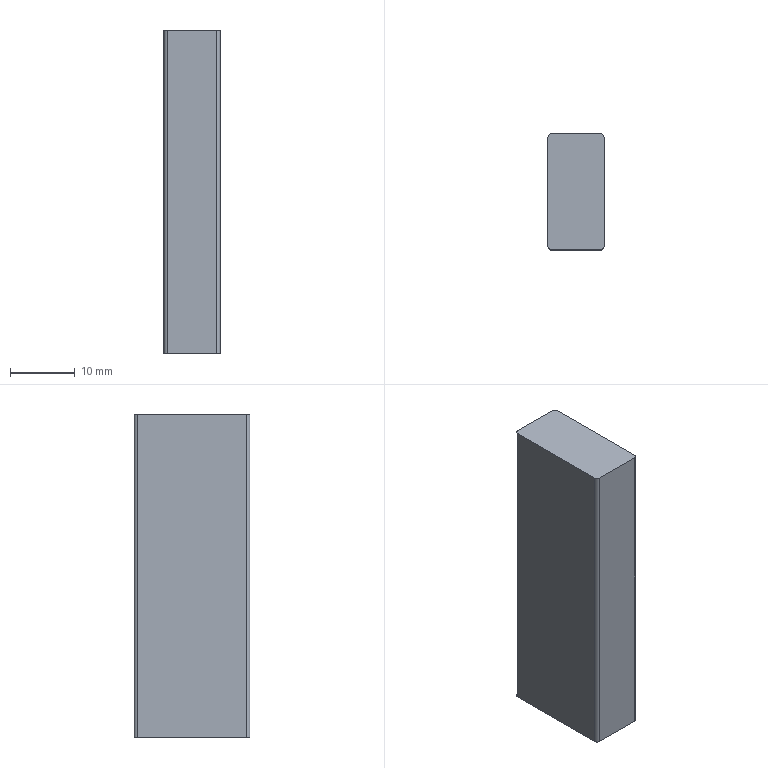Part | NX | features BREP 1 | 1 solid | 10 faces | box 8.68 x 17.946 x 50 mm | volume 7778 mm3 | plane 6 | cylinder 4 | commonest cylinder face diameters 1 x4
STEP:
#1=CARTESIAN_POINT('',(-3.84,8.973,-40.6));
#2=VERTEX_POINT('',#1);
#3=CARTESIAN_POINT('',(-4.34,8.473,-40.6));
#4=VERTEX_POINT('',#3);
#5=CARTESIAN_POINT('',(-3.84,8.473,-40.6));
#6=DIRECTION('',(0.,0.,1.));
#7=DIRECTION('',(1.,0.,0.));
#8=AXIS2_PLACEMENT_3D('',#5,#6,#7);
#9=CIRCLE('',#8,0.5);
#10=EDGE_CURVE('',#2,#4,#9,.T.);
#11=ORIENTED_EDGE('',*,*,#10,.F.);
#12=CARTESIAN_POINT('',(-3.84,8.973,-90.6));
#13=VERTEX_POINT('',#12);
#14=CARTESIAN_POINT('',(-3.84,8.973,-90.6));
#15=DIRECTION('',(0.,0.,1.));
#16=VECTOR('',#15,1000.);
#17=LINE('',#14,#16);
#18=EDGE_CURVE('',#13,#2,#17,.T.);
#19=ORIENTED_EDGE('',*,*,#18,.F.);
#20=CARTESIAN_POINT('',(-4.34,8.473,-90.6));
#21=VERTEX_POINT('',#20);
#22=CARTESIAN_POINT('',(-3.84,8.473,-90.6));
#23=DIRECTION('',(0.,0.,1.));
#24=DIRECTION('',(1.,0.,0.));
#25=AXIS2_PLACEMENT_3D('',#22,#23,#24);
#26=CIRCLE('',#25,0.5);
#27=EDGE_CURVE('',#13,#21,#26,.T.);
#28=ORIENTED_EDGE('',*,*,#27,.T.);
#29=CARTESIAN_POINT('',(-4.34,8.473,-90.6));
#30=DIRECTION('',(0.,0.,1.));
#31=VECTOR('',#30,1000.);
#32=LINE('',#29,#31);
#33=EDGE_CURVE('',#21,#4,#32,.T.);
#34=ORIENTED_EDGE('',*,*,#33,.T.);
#35=EDGE_LOOP('',(#11,#19,#28,#34));
#36=FACE_BOUND('',#35,.T.);
#37=CARTESIAN_POINT('',(-3.84,8.473,-90.6));
#38=DIRECTION('',(0.,0.,1.));
#39=DIRECTION('',(-1.,0.,0.));
#40=AXIS2_PLACEMENT_3D('',#37,#38,#39);
#41=CYLINDRICAL_SURFACE('',#40,0.5);
#42=ADVANCED_FACE('',(#36),#41,.T.);
#43=CARTESIAN_POINT('',(-4.34,-8.473,-40.6));
#44=VERTEX_POINT('',#43);
#45=CARTESIAN_POINT('',(-4.34,-8.473,-40.6));
#46=DIRECTION('',(0.,1.,0.));
#47=VECTOR('',#46,1000.);
#48=LINE('',#45,#47);
#49=EDGE_CURVE('',#44,#4,#48,.T.);
#50=ORIENTED_EDGE('',*,*,#49,.T.);
#51=ORIENTED_EDGE('',*,*,#33,.F.);
#52=CARTESIAN_POINT('',(-4.34,-8.473,-90.6));
#53=VERTEX_POINT('',#52);
#54=CARTESIAN_POINT('',(-4.34,-8.473,-90.6));
#55=DIRECTION('',(0.,1.,0.));
#56=VECTOR('',#55,1000.);
#57=LINE('',#54,#56);
#58=EDGE_CURVE('',#53,#21,#57,.T.);
#59=ORIENTED_EDGE('',*,*,#58,.F.);
#60=CARTESIAN_POINT('',(-4.34,-8.473,-90.6));
#61=DIRECTION('',(0.,0.,1.));
#62=VECTOR('',#61,1000.);
#63=LINE('',#60,#62);
#64=EDGE_CURVE('',#53,#44,#63,.T.);
#65=ORIENTED_EDGE('',*,*,#64,.T.);
#66=EDGE_LOOP('',(#50,#51,#59,#65));
#67=FACE_BOUND('',#66,.T.);
#68=CARTESIAN_POINT('',(-4.34,-8.473,-90.6));
#69=DIRECTION('',(1.,0.,0.));
#70=DIRECTION('',(0.,-1.,0.));
#71=AXIS2_PLACEMENT_3D('',#68,#69,#70);
#72=PLANE('',#71);
#73=ADVANCED_FACE('',(#67),#72,.F.);
#74=CARTESIAN_POINT('',(-3.84,-8.973,-40.6));
#75=VERTEX_POINT('',#74);
#76=CARTESIAN_POINT('',(-3.84,-8.473,-40.6));
#77=DIRECTION('',(0.,0.,1.));
#78=DIRECTION('',(1.,0.,0.));
#79=AXIS2_PLACEMENT_3D('',#76,#77,#78);
#80=CIRCLE('',#79,0.5);
#81=EDGE_CURVE('',#44,#75,#80,.T.);
#82=ORIENTED_EDGE('',*,*,#81,.F.);
#83=ORIENTED_EDGE('',*,*,#64,.F.);
#84=CARTESIAN_POINT('',(-3.84,-8.973,-90.6));
#85=VERTEX_POINT('',#84);
#86=CARTESIAN_POINT('',(-3.84,-8.473,-90.6));
#87=DIRECTION('',(0.,0.,1.));
#88=DIRECTION('',(1.,0.,0.));
#89=AXIS2_PLACEMENT_3D('',#86,#87,#88);
#90=CIRCLE('',#89,0.5);
#91=EDGE_CURVE('',#53,#85,#90,.T.);
#92=ORIENTED_EDGE('',*,*,#91,.T.);
#93=CARTESIAN_POINT('',(-3.84,-8.973,-90.6));
#94=DIRECTION('',(0.,0.,1.));
#95=VECTOR('',#94,1000.);
#96=LINE('',#93,#95);
#97=EDGE_CURVE('',#85,#75,#96,.T.);
#98=ORIENTED_EDGE('',*,*,#97,.T.);
#99=EDGE_LOOP('',(#82,#83,#92,#98));
#100=FACE_BOUND('',#99,.T.);
#101=CARTESIAN_POINT('',(-3.84,-8.473,-90.6));
#102=DIRECTION('',(0.,0.,1.));
#103=DIRECTION('',(-1.,0.,0.));
#104=AXIS2_PLACEMENT_3D('',#101,#102,#103);
#105=CYLINDRICAL_SURFACE('',#104,0.5);
#106=ADVANCED_FACE('',(#100),#105,.T.);
#107=CARTESIAN_POINT('',(3.84,-8.973,-40.6));
#108=VERTEX_POINT('',#107);
#109=CARTESIAN_POINT('',(3.84,-8.973,-40.6));
#110=DIRECTION('',(-1.,0.,0.));
#111=VECTOR('',#110,1000.);
#112=LINE('',#109,#111);
#113=EDGE_CURVE('',#108,#75,#112,.T.);
#114=ORIENTED_EDGE('',*,*,#113,.T.);
#115=ORIENTED_EDGE('',*,*,#97,.F.);
#116=CARTESIAN_POINT('',(3.84,-8.973,-90.6));
#117=VERTEX_POINT('',#116);
#118=CARTESIAN_POINT('',(3.84,-8.973,-90.6));
#119=DIRECTION('',(-1.,0.,0.));
#120=VECTOR('',#119,1000.);
#121=LINE('',#118,#120);
#122=EDGE_CURVE('',#117,#85,#121,.T.);
#123=ORIENTED_EDGE('',*,*,#122,.F.);
#124=CARTESIAN_POINT('',(3.84,-8.973,-90.6));
#125=DIRECTION('',(0.,0.,1.));
#126=VECTOR('',#125,1000.);
#127=LINE('',#124,#126);
#128=EDGE_CURVE('',#117,#108,#127,.T.);
#129=ORIENTED_EDGE('',*,*,#128,.T.);
#130=EDGE_LOOP('',(#114,#115,#123,#129));
#131=FACE_BOUND('',#130,.T.);
#132=CARTESIAN_POINT('',(3.84,-8.973,-90.6));
#133=DIRECTION('',(0.,1.,0.));
#134=DIRECTION('',(0.,0.,-1.));
#135=AXIS2_PLACEMENT_3D('',#132,#133,#134);
#136=PLANE('',#135);
#137=ADVANCED_FACE('',(#131),#136,.F.);
#138=CARTESIAN_POINT('',(4.34,-8.473,-40.6));
#139=VERTEX_POINT('',#138);
#140=CARTESIAN_POINT('',(3.84,-8.473,-40.6));
#141=DIRECTION('',(0.,0.,1.));
#142=DIRECTION('',(1.,0.,0.));
#143=AXIS2_PLACEMENT_3D('',#140,#141,#142);
#144=CIRCLE('',#143,0.5);
#145=EDGE_CURVE('',#108,#139,#144,.T.);
#146=ORIENTED_EDGE('',*,*,#145,.F.);
#147=ORIENTED_EDGE('',*,*,#128,.F.);
#148=CARTESIAN_POINT('',(4.34,-8.473,-90.6));
#149=VERTEX_POINT('',#148);
#150=CARTESIAN_POINT('',(3.84,-8.473,-90.6));
#151=DIRECTION('',(0.,0.,1.));
#152=DIRECTION('',(1.,0.,0.));
#153=AXIS2_PLACEMENT_3D('',#150,#151,#152);
#154=CIRCLE('',#153,0.5);
#155=EDGE_CURVE('',#117,#149,#154,.T.);
#156=ORIENTED_EDGE('',*,*,#155,.T.);
#157=CARTESIAN_POINT('',(4.34,-8.473,-90.6));
#158=DIRECTION('',(0.,0.,1.));
#159=VECTOR('',#158,1000.);
#160=LINE('',#157,#159);
#161=EDGE_CURVE('',#149,#139,#160,.T.);
#162=ORIENTED_EDGE('',*,*,#161,.T.);
#163=EDGE_LOOP('',(#146,#147,#156,#162));
#164=FACE_BOUND('',#163,.T.);
#165=CARTESIAN_POINT('',(3.84,-8.473,-90.6));
#166=DIRECTION('',(0.,0.,1.));
#167=DIRECTION('',(-1.,0.,0.));
#168=AXIS2_PLACEMENT_3D('',#165,#166,#167);
#169=CYLINDRICAL_SURFACE('',#168,0.5);
#170=ADVANCED_FACE('',(#164),#169,.T.);
#171=CARTESIAN_POINT('',(4.34,8.473,-40.6));
#172=VERTEX_POINT('',#171);
#173=CARTESIAN_POINT('',(4.34,8.473,-40.6));
#174=DIRECTION('',(0.,-1.,0.));
#175=VECTOR('',#174,1000.);
#176=LINE('',#173,#175);
#177=EDGE_CURVE('',#172,#139,#176,.T.);
#178=ORIENTED_EDGE('',*,*,#177,.T.);
#179=ORIENTED_EDGE('',*,*,#161,.F.);
#180=CARTESIAN_POINT('',(4.34,8.473,-90.6));
#181=VERTEX_POINT('',#180);
#182=CARTESIAN_POINT('',(4.34,8.473,-90.6));
#183=DIRECTION('',(0.,-1.,0.));
#184=VECTOR('',#183,1000.);
#185=LINE('',#182,#184);
#186=EDGE_CURVE('',#181,#149,#185,.T.);
#187=ORIENTED_EDGE('',*,*,#186,.F.);
#188=CARTESIAN_POINT('',(4.34,8.473,-90.6));
#189=DIRECTION('',(0.,0.,1.));
#190=VECTOR('',#189,1000.);
#191=LINE('',#188,#190);
#192=EDGE_CURVE('',#181,#172,#191,.T.);
#193=ORIENTED_EDGE('',*,*,#192,.T.);
#194=EDGE_LOOP('',(#178,#179,#187,#193));
#195=FACE_BOUND('',#194,.T.);
#196=CARTESIAN_POINT('',(4.34,8.473,-90.6));
#197=DIRECTION('',(-1.,0.,0.));
#198=DIRECTION('',(0.,0.,-1.));
#199=AXIS2_PLACEMENT_3D('',#196,#197,#198);
#200=PLANE('',#199);
#201=ADVANCED_FACE('',(#195),#200,.F.);
#202=CARTESIAN_POINT('',(3.84,8.973,-40.6));
#203=VERTEX_POINT('',#202);
#204=CARTESIAN_POINT('',(3.84,8.473,-40.6));
#205=DIRECTION('',(0.,0.,1.));
#206=DIRECTION('',(1.,0.,0.));
#207=AXIS2_PLACEMENT_3D('',#204,#205,#206);
#208=CIRCLE('',#207,0.5);
#209=EDGE_CURVE('',#172,#203,#208,.T.);
#210=ORIENTED_EDGE('',*,*,#209,.F.);
#211=ORIENTED_EDGE('',*,*,#192,.F.);
#212=CARTESIAN_POINT('',(3.84,8.973,-90.6));
#213=VERTEX_POINT('',#212);
#214=CARTESIAN_POINT('',(3.84,8.473,-90.6));
#215=DIRECTION('',(0.,0.,1.));
#216=DIRECTION('',(1.,0.,0.));
#217=AXIS2_PLACEMENT_3D('',#214,#215,#216);
#218=CIRCLE('',#217,0.5);
#219=EDGE_CURVE('',#181,#213,#218,.T.);
#220=ORIENTED_EDGE('',*,*,#219,.T.);
#221=CARTESIAN_POINT('',(3.84,8.973,-90.6));
#222=DIRECTION('',(0.,0.,1.));
#223=VECTOR('',#222,1000.);
#224=LINE('',#221,#223);
#225=EDGE_CURVE('',#213,#203,#224,.T.);
#226=ORIENTED_EDGE('',*,*,#225,.T.);
#227=EDGE_LOOP('',(#210,#211,#220,#226));
#228=FACE_BOUND('',#227,.T.);
#229=CARTESIAN_POINT('',(3.84,8.473,-90.6));
#230=DIRECTION('',(0.,0.,1.));
#231=DIRECTION('',(-1.,0.,0.));
#232=AXIS2_PLACEMENT_3D('',#229,#230,#231);
#233=CYLINDRICAL_SURFACE('',#232,0.5);
#234=ADVANCED_FACE('',(#228),#233,.T.);
#235=CARTESIAN_POINT('',(-3.84,8.973,-40.6));
#236=DIRECTION('',(1.,0.,0.));
#237=VECTOR('',#236,1000.);
#238=LINE('',#235,#237);
#239=EDGE_CURVE('',#2,#203,#238,.T.);
#240=ORIENTED_EDGE('',*,*,#239,.T.);
#241=ORIENTED_EDGE('',*,*,#225,.F.);
#242=CARTESIAN_POINT('',(-3.84,8.973,-90.6));
#243=DIRECTION('',(1.,0.,0.));
#244=VECTOR('',#243,1000.);
#245=LINE('',#242,#244);
#246=EDGE_CURVE('',#13,#213,#245,.T.);
#247=ORIENTED_EDGE('',*,*,#246,.F.);
#248=ORIENTED_EDGE('',*,*,#18,.T.);
#249=EDGE_LOOP('',(#240,#241,#247,#248));
#250=FACE_BOUND('',#249,.T.);
#251=CARTESIAN_POINT('',(-3.84,8.973,-90.6));
#252=DIRECTION('',(0.,-1.,0.));
#253=DIRECTION('',(-1.,0.,0.));
#254=AXIS2_PLACEMENT_3D('',#251,#252,#253);
#255=PLANE('',#254);
#256=ADVANCED_FACE('',(#250),#255,.F.);
#257=ORIENTED_EDGE('',*,*,#27,.F.);
#258=ORIENTED_EDGE('',*,*,#246,.T.);
#259=ORIENTED_EDGE('',*,*,#219,.F.);
#260=ORIENTED_EDGE('',*,*,#186,.T.);
#261=ORIENTED_EDGE('',*,*,#155,.F.);
#262=ORIENTED_EDGE('',*,*,#122,.T.);
#263=ORIENTED_EDGE('',*,*,#91,.F.);
#264=ORIENTED_EDGE('',*,*,#58,.T.);
#265=EDGE_LOOP('',(#257,#258,#259,#260,#261,#262,#263,#264));
#266=FACE_BOUND('',#265,.T.);
#267=CARTESIAN_POINT('',(-3.84,8.473,-90.6));
#268=DIRECTION('',(0.,0.,1.));
#269=DIRECTION('',(-1.,0.,0.));
#270=AXIS2_PLACEMENT_3D('',#267,#268,#269);
#271=PLANE('',#270);
#272=ADVANCED_FACE('',(#266),#271,.F.);
#273=ORIENTED_EDGE('',*,*,#10,.T.);
#274=ORIENTED_EDGE('',*,*,#49,.F.);
#275=ORIENTED_EDGE('',*,*,#81,.T.);
#276=ORIENTED_EDGE('',*,*,#113,.F.);
#277=ORIENTED_EDGE('',*,*,#145,.T.);
#278=ORIENTED_EDGE('',*,*,#177,.F.);
#279=ORIENTED_EDGE('',*,*,#209,.T.);
#280=ORIENTED_EDGE('',*,*,#239,.F.);
#281=EDGE_LOOP('',(#273,#274,#275,#276,#277,#278,#279,#280));
#282=FACE_BOUND('',#281,.T.);
#283=CARTESIAN_POINT('',(-3.84,8.473,-40.6));
#284=DIRECTION('',(0.,0.,1.));
#285=DIRECTION('',(-1.,0.,0.));
#286=AXIS2_PLACEMENT_3D('',#283,#284,#285);
#287=PLANE('',#286);
#288=ADVANCED_FACE('',(#282),#287,.T.);
#289=CLOSED_SHELL('',(#42,#73,#106,#137,#170,#201,#234,#256,#272,#288));
#290=MANIFOLD_SOLID_BREP('',#289);
#291=(LENGTH_UNIT()NAMED_UNIT(*)SI_UNIT(.MILLI.,.METRE.));
#292=UNCERTAINTY_MEASURE_WITH_UNIT(LENGTH_MEASURE(0.00001),#291,'','');
#293=(NAMED_UNIT(*)PLANE_ANGLE_UNIT()SI_UNIT($,.RADIAN.));
#294=(NAMED_UNIT(*)SI_UNIT($,.STERADIAN.)SOLID_ANGLE_UNIT());
#295=(GEOMETRIC_REPRESENTATION_CONTEXT(3)GLOBAL_UNCERTAINTY_ASSIGNED_CONTEXT((#292))GLOBAL_UNIT_ASSIGNED_CONTEXT((#291,#293,#294))REPRESENTATION_CONTEXT('',''));
#296=ADVANCED_BREP_SHAPE_REPRESENTATION('',(#290),#295);